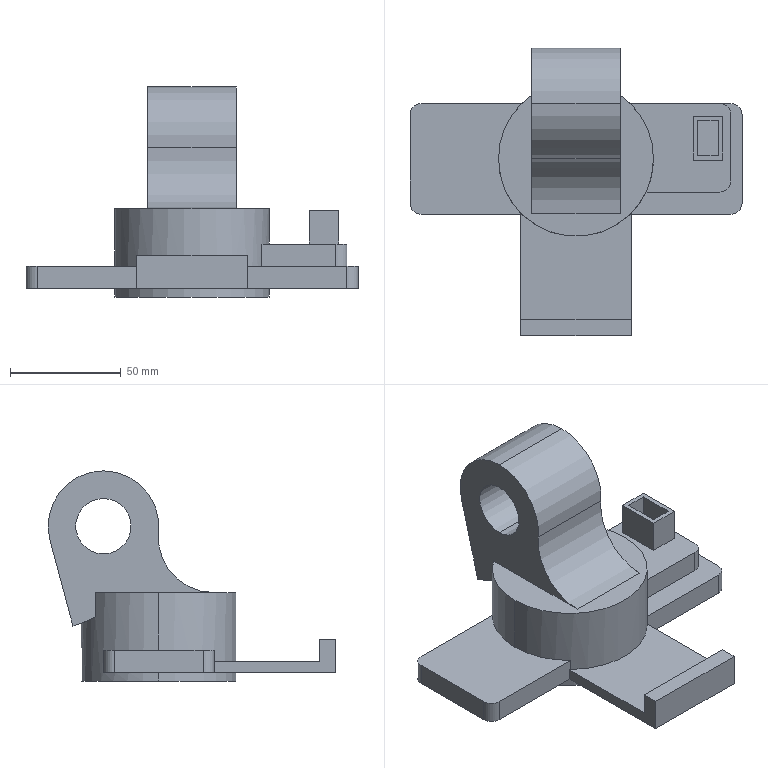Part | SolidWorks | features ICE 6, Fillet 4, Cut 2, Extrusion 1 | 1 solid | 48 faces | box 150 x 130 x 95 mm | volume 315540 mm3 | plane 33 | cylinder 15 | commonest cylinder face diameters 10 x6 50 x3 70 x3 25 x2 80 x1
STEP:
#1=CARTESIAN_POINT('',(-20.,25.,82.5));
#2=VERTEX_POINT('',#1);
#3=CARTESIAN_POINT('',(-20.,25.,57.5));
#4=VERTEX_POINT('',#3);
#5=CARTESIAN_POINT('',(-20.,25.,70.));
#6=DIRECTION('',(1.,0.,0.));
#7=DIRECTION('',(0.,0.,-1.));
#8=AXIS2_PLACEMENT_3D('',#5,#6,#7);
#9=CIRCLE('',#8,12.5);
#10=EDGE_CURVE('',#2,#4,#9,.T.);
#11=ORIENTED_EDGE('',*,*,#10,.F.);
#12=CARTESIAN_POINT('',(20.,25.,82.5));
#13=VERTEX_POINT('',#12);
#14=CARTESIAN_POINT('',(-75.,25.,82.5));
#15=DIRECTION('',(1.,0.,0.));
#16=VECTOR('',#15,1000.);
#17=LINE('',#14,#16);
#18=EDGE_CURVE('',#2,#13,#17,.T.);
#19=ORIENTED_EDGE('',*,*,#18,.T.);
#20=CARTESIAN_POINT('',(20.,25.,57.5));
#21=VERTEX_POINT('',#20);
#22=CARTESIAN_POINT('',(20.,25.,70.));
#23=DIRECTION('',(1.,0.,0.));
#24=DIRECTION('',(0.,0.,-1.));
#25=AXIS2_PLACEMENT_3D('',#22,#23,#24);
#26=CIRCLE('',#25,12.5);
#27=EDGE_CURVE('',#13,#21,#26,.T.);
#28=ORIENTED_EDGE('',*,*,#27,.T.);
#29=CARTESIAN_POINT('',(-75.,25.,57.5));
#30=DIRECTION('',(1.,0.,0.));
#31=VECTOR('',#30,1000.);
#32=LINE('',#29,#31);
#33=EDGE_CURVE('',#4,#21,#32,.T.);
#34=ORIENTED_EDGE('',*,*,#33,.F.);
#35=EDGE_LOOP('',(#11,#19,#28,#34));
#36=FACE_OUTER_BOUND('',#35,.T.);
#37=CARTESIAN_POINT('',(-75.,25.,70.));
#38=DIRECTION('',(1.,0.,0.));
#39=DIRECTION('',(0.,0.,-1.));
#40=AXIS2_PLACEMENT_3D('',#37,#38,#39);
#41=CYLINDRICAL_SURFACE('',#40,12.5);
#42=ADVANCED_FACE('',(#36),#41,.F.);
#43=CARTESIAN_POINT('',(20.,25.,95.));
#44=VERTEX_POINT('',#43);
#45=CARTESIAN_POINT('',(20.,0.1253,67.5));
#46=VERTEX_POINT('',#45);
#47=CARTESIAN_POINT('',(20.,25.,70.));
#48=DIRECTION('',(1.,0.,0.));
#49=DIRECTION('',(0.,0.,-1.));
#50=AXIS2_PLACEMENT_3D('',#47,#48,#49);
#51=CIRCLE('',#50,25.);
#52=EDGE_CURVE('',#44,#46,#51,.T.);
#53=ORIENTED_EDGE('',*,*,#52,.F.);
#54=CARTESIAN_POINT('',(-20.,25.,95.));
#55=VERTEX_POINT('',#54);
#56=CARTESIAN_POINT('',(20.,25.,95.));
#57=DIRECTION('',(-1.,0.,0.));
#58=VECTOR('',#57,1000.);
#59=LINE('',#56,#58);
#60=EDGE_CURVE('',#44,#55,#59,.T.);
#61=ORIENTED_EDGE('',*,*,#60,.T.);
#62=CARTESIAN_POINT('',(-20.,0.1253,67.5));
#63=VERTEX_POINT('',#62);
#64=CARTESIAN_POINT('',(-20.,25.,70.));
#65=DIRECTION('',(1.,0.,0.));
#66=DIRECTION('',(0.,0.,-1.));
#67=AXIS2_PLACEMENT_3D('',#64,#65,#66);
#68=CIRCLE('',#67,25.);
#69=EDGE_CURVE('',#55,#63,#68,.T.);
#70=ORIENTED_EDGE('',*,*,#69,.T.);
#71=CARTESIAN_POINT('',(20.,0.1253,67.5));
#72=DIRECTION('',(1.,0.,0.));
#73=VECTOR('',#72,1000.);
#74=LINE('',#71,#73);
#75=EDGE_CURVE('',#63,#46,#74,.T.);
#76=ORIENTED_EDGE('',*,*,#75,.T.);
#77=EDGE_LOOP('',(#53,#61,#70,#76));
#78=FACE_OUTER_BOUND('',#77,.T.);
#79=CARTESIAN_POINT('',(20.,25.,70.));
#80=DIRECTION('',(-1.,0.,0.));
#81=DIRECTION('',(0.,0.,1.));
#82=AXIS2_PLACEMENT_3D('',#79,#80,#81);
#83=CYLINDRICAL_SURFACE('',#82,25.);
#84=ADVANCED_FACE('',(#78),#83,.T.);
#85=CARTESIAN_POINT('',(35.,0.,40.));
#86=VERTEX_POINT('',#85);
#87=CARTESIAN_POINT('',(20.,28.723,40.));
#88=VERTEX_POINT('',#87);
#89=CARTESIAN_POINT('',(0.,0.,40.));
#90=DIRECTION('',(0.,0.,1.));
#91=DIRECTION('',(1.,0.,0.));
#92=AXIS2_PLACEMENT_3D('',#89,#90,#91);
#93=CIRCLE('',#92,35.);
#94=EDGE_CURVE('',#86,#88,#93,.T.);
#95=ORIENTED_EDGE('',*,*,#94,.F.);
#96=CARTESIAN_POINT('',(35.,0.,24.));
#97=VERTEX_POINT('',#96);
#98=CARTESIAN_POINT('',(35.,0.,40.));
#99=DIRECTION('',(0.,0.,-1.));
#100=VECTOR('',#99,1000.);
#101=LINE('',#98,#100);
#102=EDGE_CURVE('',#86,#97,#101,.T.);
#103=ORIENTED_EDGE('',*,*,#102,.T.);
#104=CARTESIAN_POINT('',(24.495,25.,24.));
#105=VERTEX_POINT('',#104);
#106=CARTESIAN_POINT('',(0.,0.,24.));
#107=DIRECTION('',(0.,0.,-1.));
#108=DIRECTION('',(0.,1.,0.));
#109=AXIS2_PLACEMENT_3D('',#106,#107,#108);
#110=CIRCLE('',#109,35.);
#111=EDGE_CURVE('',#105,#97,#110,.T.);
#112=ORIENTED_EDGE('',*,*,#111,.F.);
#113=CARTESIAN_POINT('',(24.495,25.,4.));
#114=VERTEX_POINT('',#113);
#115=CARTESIAN_POINT('',(24.495,25.,40.));
#116=DIRECTION('',(0.,0.,1.));
#117=VECTOR('',#116,1000.);
#118=LINE('',#115,#117);
#119=EDGE_CURVE('',#114,#105,#118,.T.);
#120=ORIENTED_EDGE('',*,*,#119,.F.);
#121=CARTESIAN_POINT('',(35.,0.,4.));
#122=VERTEX_POINT('',#121);
#123=CARTESIAN_POINT('',(0.,0.,4.));
#124=DIRECTION('',(0.,0.,-1.));
#125=DIRECTION('',(-1.,0.,0.));
#126=AXIS2_PLACEMENT_3D('',#123,#124,#125);
#127=CIRCLE('',#126,35.);
#128=EDGE_CURVE('',#114,#122,#127,.T.);
#129=ORIENTED_EDGE('',*,*,#128,.T.);
#130=CARTESIAN_POINT('',(35.,0.,0.));
#131=VERTEX_POINT('',#130);
#132=CARTESIAN_POINT('',(35.,0.,40.));
#133=DIRECTION('',(0.,0.,-1.));
#134=VECTOR('',#133,1000.);
#135=LINE('',#132,#134);
#136=EDGE_CURVE('',#122,#131,#135,.T.);
#137=ORIENTED_EDGE('',*,*,#136,.T.);
#138=CARTESIAN_POINT('',(-35.,0.,0.));
#139=VERTEX_POINT('',#138);
#140=CARTESIAN_POINT('',(0.,0.,0.));
#141=DIRECTION('',(0.,0.,1.));
#142=DIRECTION('',(1.,0.,0.));
#143=AXIS2_PLACEMENT_3D('',#140,#141,#142);
#144=CIRCLE('',#143,35.);
#145=EDGE_CURVE('',#131,#139,#144,.T.);
#146=ORIENTED_EDGE('',*,*,#145,.T.);
#147=CARTESIAN_POINT('',(-35.,0.,4.));
#148=VERTEX_POINT('',#147);
#149=CARTESIAN_POINT('',(-35.,0.,40.));
#150=DIRECTION('',(0.,0.,-1.));
#151=VECTOR('',#150,1000.);
#152=LINE('',#149,#151);
#153=EDGE_CURVE('',#148,#139,#152,.T.);
#154=ORIENTED_EDGE('',*,*,#153,.F.);
#155=CARTESIAN_POINT('',(-24.495,25.,4.));
#156=VERTEX_POINT('',#155);
#157=CARTESIAN_POINT('',(0.,0.,4.));
#158=DIRECTION('',(0.,0.,-1.));
#159=DIRECTION('',(-1.,0.,0.));
#160=AXIS2_PLACEMENT_3D('',#157,#158,#159);
#161=CIRCLE('',#160,35.);
#162=EDGE_CURVE('',#148,#156,#161,.T.);
#163=ORIENTED_EDGE('',*,*,#162,.T.);
#164=CARTESIAN_POINT('',(-24.495,25.,14.));
#165=VERTEX_POINT('',#164);
#166=CARTESIAN_POINT('',(-24.495,25.,40.));
#167=DIRECTION('',(0.,0.,-1.));
#168=VECTOR('',#167,1000.);
#169=LINE('',#166,#168);
#170=EDGE_CURVE('',#165,#156,#169,.T.);
#171=ORIENTED_EDGE('',*,*,#170,.F.);
#172=CARTESIAN_POINT('',(-35.,0.,14.));
#173=VERTEX_POINT('',#172);
#174=CARTESIAN_POINT('',(0.,0.,14.));
#175=DIRECTION('',(0.,0.,-1.));
#176=DIRECTION('',(0.,1.,0.));
#177=AXIS2_PLACEMENT_3D('',#174,#175,#176);
#178=CIRCLE('',#177,35.);
#179=EDGE_CURVE('',#173,#165,#178,.T.);
#180=ORIENTED_EDGE('',*,*,#179,.F.);
#181=CARTESIAN_POINT('',(-35.,0.,40.));
#182=VERTEX_POINT('',#181);
#183=CARTESIAN_POINT('',(-35.,0.,40.));
#184=DIRECTION('',(0.,0.,-1.));
#185=VECTOR('',#184,1000.);
#186=LINE('',#183,#185);
#187=EDGE_CURVE('',#182,#173,#186,.T.);
#188=ORIENTED_EDGE('',*,*,#187,.F.);
#189=CARTESIAN_POINT('',(-20.,28.723,40.));
#190=VERTEX_POINT('',#189);
#191=CARTESIAN_POINT('',(0.,0.,40.));
#192=DIRECTION('',(0.,0.,1.));
#193=DIRECTION('',(1.,0.,0.));
#194=AXIS2_PLACEMENT_3D('',#191,#192,#193);
#195=CIRCLE('',#194,35.);
#196=EDGE_CURVE('',#190,#182,#195,.T.);
#197=ORIENTED_EDGE('',*,*,#196,.F.);
#198=CARTESIAN_POINT('',(-20.,28.723,29.138));
#199=VERTEX_POINT('',#198);
#200=CARTESIAN_POINT('',(-20.,28.723,40.));
#201=DIRECTION('',(0.,0.,1.));
#202=VECTOR('',#201,1000.);
#203=LINE('',#200,#202);
#204=EDGE_CURVE('',#199,#190,#203,.T.);
#205=ORIENTED_EDGE('',*,*,#204,.F.);
#206=CARTESIAN_POINT('',(20.,28.723,29.138));
#207=VERTEX_POINT('',#206);
#208=CARTESIAN_POINT('',(20.,28.723,29.138));
#209=CARTESIAN_POINT('',(19.295,29.214,28.846));
#210=CARTESIAN_POINT('',(18.566,29.682,28.582));
#211=CARTESIAN_POINT('',(17.074,30.565,28.105));
#212=CARTESIAN_POINT('',(16.308,30.981,27.89));
#213=CARTESIAN_POINT('',(14.738,31.758,27.505));
#214=CARTESIAN_POINT('',(13.933,32.119,27.333));
#215=CARTESIAN_POINT('',(12.286,32.785,27.028));
#216=CARTESIAN_POINT('',(11.439,33.09,26.893));
#217=CARTESIAN_POINT('',(8.876,33.903,26.544));
#218=CARTESIAN_POINT('',(7.136,34.312,26.382));
#219=CARTESIAN_POINT('',(4.482,34.723,26.221));
#220=CARTESIAN_POINT('',(3.589,34.827,26.181));
#221=CARTESIAN_POINT('',(1.79,34.966,26.128));
#222=CARTESIAN_POINT('',(0.8798,35.001,26.115));
#223=CARTESIAN_POINT('',(-1.825,34.999,26.116));
#224=CARTESIAN_POINT('',(-3.61,34.859,26.168));
#225=CARTESIAN_POINT('',(-6.261,34.447,26.329));
#226=CARTESIAN_POINT('',(-7.14,34.276,26.397));
#227=CARTESIAN_POINT('',(-8.89,33.864,26.564));
#228=CARTESIAN_POINT('',(-9.762,33.623,26.664));
#229=CARTESIAN_POINT('',(-12.318,32.809,27.014));
#230=CARTESIAN_POINT('',(-13.954,32.146,27.313));
#231=CARTESIAN_POINT('',(-16.303,30.984,27.889));
#232=CARTESIAN_POINT('',(-17.069,30.568,28.103));
#233=CARTESIAN_POINT('',(-18.565,29.683,28.581));
#234=CARTESIAN_POINT('',(-19.298,29.211,28.847));
#235=CARTESIAN_POINT('',(-20.,28.723,29.138));
#236=B_SPLINE_CURVE_WITH_KNOTS('',3,(#208,#209,#210,#211,#212,#213,#214,#215,#216,#217,#218,#219,#220,#221,#222,#223,#224,#225,#226,#227,#228,#229,#230,#231,#232,#233,#234,#235),.UNSPECIFIED.,.F.,.F.,(4,2,2,2,2,2,2,2,2,2,2,2,2,4),(0.01965,0.02233,0.02502,0.02771,0.03039,0.03577,0.03846,0.04114,0.04652,0.0492,0.05189,0.05726,0.05995,0.06264),.UNSPECIFIED.);
#237=EDGE_CURVE('',#207,#199,#236,.T.);
#238=ORIENTED_EDGE('',*,*,#237,.F.);
#239=CARTESIAN_POINT('',(20.,28.723,40.));
#240=DIRECTION('',(0.,0.,1.));
#241=VECTOR('',#240,1000.);
#242=LINE('',#239,#241);
#243=EDGE_CURVE('',#207,#88,#242,.T.);
#244=ORIENTED_EDGE('',*,*,#243,.T.);
#245=EDGE_LOOP('',(#95,#103,#112,#120,#129,#137,#146,#154,#163,#171,#180,#188,#197,#205,#238,#244));
#246=FACE_OUTER_BOUND('',#245,.T.);
#247=CARTESIAN_POINT('',(0.,0.,40.));
#248=DIRECTION('',(0.,0.,-1.));
#249=DIRECTION('',(-1.,0.,0.));
#250=AXIS2_PLACEMENT_3D('',#247,#248,#249);
#251=CYLINDRICAL_SURFACE('',#250,35.);
#252=ADVANCED_FACE('',(#246),#251,.T.);
#253=ORIENTED_EDGE('',*,*,#102,.F.);
#254=CARTESIAN_POINT('',(0.,0.,40.));
#255=DIRECTION('',(0.,0.,1.));
#256=DIRECTION('',(1.,0.,0.));
#257=AXIS2_PLACEMENT_3D('',#254,#255,#256);
#258=CIRCLE('',#257,35.);
#259=EDGE_CURVE('',#182,#86,#258,.T.);
#260=ORIENTED_EDGE('',*,*,#259,.F.);
#261=ORIENTED_EDGE('',*,*,#187,.T.);
#262=CARTESIAN_POINT('',(-24.495,-25.,14.));
#263=VERTEX_POINT('',#262);
#264=CARTESIAN_POINT('',(0.,0.,14.));
#265=DIRECTION('',(0.,0.,-1.));
#266=DIRECTION('',(0.,1.,0.));
#267=AXIS2_PLACEMENT_3D('',#264,#265,#266);
#268=CIRCLE('',#267,35.);
#269=EDGE_CURVE('',#263,#173,#268,.T.);
#270=ORIENTED_EDGE('',*,*,#269,.F.);
#271=CARTESIAN_POINT('',(-24.495,-25.,9.));
#272=VERTEX_POINT('',#271);
#273=CARTESIAN_POINT('',(-24.495,-25.,40.));
#274=DIRECTION('',(0.,0.,1.));
#275=VECTOR('',#274,1000.);
#276=LINE('',#273,#275);
#277=EDGE_CURVE('',#272,#263,#276,.T.);
#278=ORIENTED_EDGE('',*,*,#277,.F.);
#279=CARTESIAN_POINT('',(24.495,-25.,9.));
#280=VERTEX_POINT('',#279);
#281=CARTESIAN_POINT('',(0.,0.,9.));
#282=DIRECTION('',(0.,0.,1.));
#283=DIRECTION('',(1.,0.,0.));
#284=AXIS2_PLACEMENT_3D('',#281,#282,#283);
#285=CIRCLE('',#284,35.);
#286=EDGE_CURVE('',#272,#280,#285,.T.);
#287=ORIENTED_EDGE('',*,*,#286,.T.);
#288=CARTESIAN_POINT('',(24.495,-25.,14.));
#289=VERTEX_POINT('',#288);
#290=CARTESIAN_POINT('',(24.495,-25.,40.));
#291=DIRECTION('',(0.,0.,-1.));
#292=VECTOR('',#291,1000.);
#293=LINE('',#290,#292);
#294=EDGE_CURVE('',#289,#280,#293,.T.);
#295=ORIENTED_EDGE('',*,*,#294,.F.);
#296=CARTESIAN_POINT('',(31.623,-15.,14.));
#297=VERTEX_POINT('',#296);
#298=CARTESIAN_POINT('',(0.,0.,14.));
#299=DIRECTION('',(0.,0.,-1.));
#300=DIRECTION('',(0.,1.,0.));
#301=AXIS2_PLACEMENT_3D('',#298,#299,#300);
#302=CIRCLE('',#301,35.);
#303=EDGE_CURVE('',#297,#289,#302,.T.);
#304=ORIENTED_EDGE('',*,*,#303,.F.);
#305=CARTESIAN_POINT('',(31.623,-15.,24.));
#306=VERTEX_POINT('',#305);
#307=CARTESIAN_POINT('',(31.623,-15.,40.));
#308=DIRECTION('',(0.,0.,-1.));
#309=VECTOR('',#308,1000.);
#310=LINE('',#307,#309);
#311=EDGE_CURVE('',#306,#297,#310,.T.);
#312=ORIENTED_EDGE('',*,*,#311,.F.);
#313=CARTESIAN_POINT('',(0.,0.,24.));
#314=DIRECTION('',(0.,0.,-1.));
#315=DIRECTION('',(0.,1.,0.));
#316=AXIS2_PLACEMENT_3D('',#313,#314,#315);
#317=CIRCLE('',#316,35.);
#318=EDGE_CURVE('',#97,#306,#317,.T.);
#319=ORIENTED_EDGE('',*,*,#318,.F.);
#320=EDGE_LOOP('',(#253,#260,#261,#270,#278,#287,#295,#304,#312,#319));
#321=FACE_OUTER_BOUND('',#320,.T.);
#322=CARTESIAN_POINT('',(0.,0.,40.));
#323=DIRECTION('',(0.,0.,-1.));
#324=DIRECTION('',(-1.,0.,0.));
#325=AXIS2_PLACEMENT_3D('',#322,#323,#324);
#326=CYLINDRICAL_SURFACE('',#325,35.);
#327=ADVANCED_FACE('',(#321),#326,.T.);
#328=CARTESIAN_POINT('',(65.,-15.,24.));
#329=VERTEX_POINT('',#328);
#330=CARTESIAN_POINT('',(70.,-15.,24.));
#331=DIRECTION('',(-1.,0.,0.));
#332=VECTOR('',#331,1000.);
#333=LINE('',#330,#332);
#334=EDGE_CURVE('',#329,#306,#333,.T.);
#335=ORIENTED_EDGE('',*,*,#334,.F.);
#336=CARTESIAN_POINT('',(70.,-10.,24.));
#337=VERTEX_POINT('',#336);
#338=CARTESIAN_POINT('',(65.,-10.,24.));
#339=DIRECTION('',(0.,0.,1.));
#340=DIRECTION('',(0.,1.,0.));
#341=AXIS2_PLACEMENT_3D('',#338,#339,#340);
#342=CIRCLE('',#341,5.);
#343=EDGE_CURVE('',#329,#337,#342,.T.);
#344=ORIENTED_EDGE('',*,*,#343,.T.);
#345=CARTESIAN_POINT('',(70.,20.,24.));
#346=VERTEX_POINT('',#345);
#347=CARTESIAN_POINT('',(70.,25.,24.));
#348=DIRECTION('',(0.,-1.,0.));
#349=VECTOR('',#348,1000.);
#350=LINE('',#347,#349);
#351=EDGE_CURVE('',#346,#337,#350,.T.);
#352=ORIENTED_EDGE('',*,*,#351,.F.);
#353=CARTESIAN_POINT('',(65.,25.,24.));
#354=VERTEX_POINT('',#353);
#355=CARTESIAN_POINT('',(65.,20.,24.));
#356=DIRECTION('',(0.,0.,1.));
#357=DIRECTION('',(0.,1.,0.));
#358=AXIS2_PLACEMENT_3D('',#355,#356,#357);
#359=CIRCLE('',#358,5.);
#360=EDGE_CURVE('',#346,#354,#359,.T.);
#361=ORIENTED_EDGE('',*,*,#360,.T.);
#362=CARTESIAN_POINT('',(70.,25.,24.));
#363=DIRECTION('',(-1.,0.,0.));
#364=VECTOR('',#363,1000.);
#365=LINE('',#362,#364);
#366=EDGE_CURVE('',#354,#105,#365,.T.);
#367=ORIENTED_EDGE('',*,*,#366,.T.);
#368=ORIENTED_EDGE('',*,*,#111,.T.);
#369=ORIENTED_EDGE('',*,*,#318,.T.);
#370=EDGE_LOOP('',(#335,#344,#352,#361,#367,#368,#369));
#371=FACE_OUTER_BOUND('',#370,.T.);
#372=CARTESIAN_POINT('',(52.886,19.241,24.));
#373=VERTEX_POINT('',#372);
#374=CARTESIAN_POINT('',(52.886,-0.6252,24.));
#375=VERTEX_POINT('',#374);
#376=CARTESIAN_POINT('',(52.886,19.241,24.));
#377=DIRECTION('',(0.,-1.,0.));
#378=VECTOR('',#377,1000.);
#379=LINE('',#376,#378);
#380=EDGE_CURVE('',#373,#375,#379,.T.);
#381=ORIENTED_EDGE('',*,*,#380,.F.);
#382=CARTESIAN_POINT('',(66.302,19.241,24.));
#383=VERTEX_POINT('',#382);
#384=CARTESIAN_POINT('',(66.302,19.241,24.));
#385=DIRECTION('',(-1.,0.,0.));
#386=VECTOR('',#385,1000.);
#387=LINE('',#384,#386);
#388=EDGE_CURVE('',#383,#373,#387,.T.);
#389=ORIENTED_EDGE('',*,*,#388,.F.);
#390=CARTESIAN_POINT('',(66.302,-0.6252,24.));
#391=VERTEX_POINT('',#390);
#392=CARTESIAN_POINT('',(66.302,19.241,24.));
#393=DIRECTION('',(0.,1.,0.));
#394=VECTOR('',#393,1000.);
#395=LINE('',#392,#394);
#396=EDGE_CURVE('',#391,#383,#395,.T.);
#397=ORIENTED_EDGE('',*,*,#396,.F.);
#398=CARTESIAN_POINT('',(66.302,-0.6252,24.));
#399=DIRECTION('',(1.,0.,0.));
#400=VECTOR('',#399,1000.);
#401=LINE('',#398,#400);
#402=EDGE_CURVE('',#375,#391,#401,.T.);
#403=ORIENTED_EDGE('',*,*,#402,.F.);
#404=EDGE_LOOP('',(#381,#389,#397,#403));
#405=FACE_BOUND('',#404,.T.);
#406=CARTESIAN_POINT('',(70.,25.,24.));
#407=DIRECTION('',(0.,0.,-1.));
#408=DIRECTION('',(0.,1.,0.));
#409=AXIS2_PLACEMENT_3D('',#406,#407,#408);
#410=PLANE('',#409);
#411=ADVANCED_FACE('',(#371,#405),#410,.F.);
#412=ORIENTED_EDGE('',*,*,#136,.F.);
#413=CARTESIAN_POINT('',(0.,0.,4.));
#414=DIRECTION('',(0.,0.,-1.));
#415=DIRECTION('',(-1.,0.,0.));
#416=AXIS2_PLACEMENT_3D('',#413,#414,#415);
#417=CIRCLE('',#416,35.);
#418=EDGE_CURVE('',#122,#148,#417,.T.);
#419=ORIENTED_EDGE('',*,*,#418,.T.);
#420=ORIENTED_EDGE('',*,*,#153,.T.);
#421=CARTESIAN_POINT('',(0.,0.,0.));
#422=DIRECTION('',(0.,0.,1.));
#423=DIRECTION('',(1.,0.,0.));
#424=AXIS2_PLACEMENT_3D('',#421,#422,#423);
#425=CIRCLE('',#424,35.);
#426=EDGE_CURVE('',#139,#131,#425,.T.);
#427=ORIENTED_EDGE('',*,*,#426,.T.);
#428=EDGE_LOOP('',(#412,#419,#420,#427));
#429=FACE_OUTER_BOUND('',#428,.T.);
#430=CARTESIAN_POINT('',(0.,0.,40.));
#431=DIRECTION('',(0.,0.,-1.));
#432=DIRECTION('',(-1.,0.,0.));
#433=AXIS2_PLACEMENT_3D('',#430,#431,#432);
#434=CYLINDRICAL_SURFACE('',#433,35.);
#435=ADVANCED_FACE('',(#429),#434,.T.);
#436=CARTESIAN_POINT('',(70.,-25.,14.));
#437=VERTEX_POINT('',#436);
#438=CARTESIAN_POINT('',(75.,-25.,14.));
#439=DIRECTION('',(-1.,0.,0.));
#440=VECTOR('',#439,1000.);
#441=LINE('',#438,#440);
#442=EDGE_CURVE('',#437,#289,#441,.T.);
#443=ORIENTED_EDGE('',*,*,#442,.F.);
#444=CARTESIAN_POINT('',(75.,-20.,14.));
#445=VERTEX_POINT('',#444);
#446=CARTESIAN_POINT('',(70.,-20.,14.));
#447=DIRECTION('',(0.,0.,1.));
#448=DIRECTION('',(0.,1.,0.));
#449=AXIS2_PLACEMENT_3D('',#446,#447,#448);
#450=CIRCLE('',#449,5.);
#451=EDGE_CURVE('',#437,#445,#450,.T.);
#452=ORIENTED_EDGE('',*,*,#451,.T.);
#453=CARTESIAN_POINT('',(75.,20.,14.));
#454=VERTEX_POINT('',#453);
#455=CARTESIAN_POINT('',(75.,25.,14.));
#456=DIRECTION('',(0.,-1.,0.));
#457=VECTOR('',#456,1000.);
#458=LINE('',#455,#457);
#459=EDGE_CURVE('',#454,#445,#458,.T.);
#460=ORIENTED_EDGE('',*,*,#459,.F.);
#461=CARTESIAN_POINT('',(70.,25.,14.));
#462=VERTEX_POINT('',#461);
#463=CARTESIAN_POINT('',(70.,20.,14.));
#464=DIRECTION('',(0.,0.,1.));
#465=DIRECTION('',(0.,1.,0.));
#466=AXIS2_PLACEMENT_3D('',#463,#464,#465);
#467=CIRCLE('',#466,5.);
#468=EDGE_CURVE('',#454,#462,#467,.T.);
#469=ORIENTED_EDGE('',*,*,#468,.T.);
#470=CARTESIAN_POINT('',(65.,25.,14.));
#471=VERTEX_POINT('',#470);
#472=CARTESIAN_POINT('',(75.,25.,14.));
#473=DIRECTION('',(1.,0.,0.));
#474=VECTOR('',#473,1000.);
#475=LINE('',#472,#474);
#476=EDGE_CURVE('',#471,#462,#475,.T.);
#477=ORIENTED_EDGE('',*,*,#476,.F.);
#478=CARTESIAN_POINT('',(70.,20.,14.));
#479=VERTEX_POINT('',#478);
#480=CARTESIAN_POINT('',(65.,20.,14.));
#481=DIRECTION('',(0.,0.,-1.));
#482=DIRECTION('',(0.,1.,0.));
#483=AXIS2_PLACEMENT_3D('',#480,#481,#482);
#484=CIRCLE('',#483,5.);
#485=EDGE_CURVE('',#471,#479,#484,.T.);
#486=ORIENTED_EDGE('',*,*,#485,.T.);
#487=CARTESIAN_POINT('',(70.,-10.,14.));
#488=VERTEX_POINT('',#487);
#489=CARTESIAN_POINT('',(70.,25.,14.));
#490=DIRECTION('',(0.,1.,0.));
#491=VECTOR('',#490,1000.);
#492=LINE('',#489,#491);
#493=EDGE_CURVE('',#488,#479,#492,.T.);
#494=ORIENTED_EDGE('',*,*,#493,.F.);
#495=CARTESIAN_POINT('',(65.,-15.,14.));
#496=VERTEX_POINT('',#495);
#497=CARTESIAN_POINT('',(65.,-10.,14.));
#498=DIRECTION('',(0.,0.,-1.));
#499=DIRECTION('',(0.,1.,0.));
#500=AXIS2_PLACEMENT_3D('',#497,#498,#499);
#501=CIRCLE('',#500,5.);
#502=EDGE_CURVE('',#488,#496,#501,.T.);
#503=ORIENTED_EDGE('',*,*,#502,.T.);
#504=CARTESIAN_POINT('',(70.,-15.,14.));
#505=DIRECTION('',(-1.,0.,0.));
#506=VECTOR('',#505,1000.);
#507=LINE('',#504,#506);
#508=EDGE_CURVE('',#496,#297,#507,.T.);
#509=ORIENTED_EDGE('',*,*,#508,.T.);
#510=ORIENTED_EDGE('',*,*,#303,.T.);
#511=EDGE_LOOP('',(#443,#452,#460,#469,#477,#486,#494,#503,#509,#510));
#512=FACE_OUTER_BOUND('',#511,.T.);
#513=CARTESIAN_POINT('',(75.,25.,14.));
#514=DIRECTION('',(0.,0.,-1.));
#515=DIRECTION('',(0.,1.,0.));
#516=AXIS2_PLACEMENT_3D('',#513,#514,#515);
#517=PLANE('',#516);
#518=ADVANCED_FACE('',(#512),#517,.F.);
#519=CARTESIAN_POINT('',(25.,-72.5,9.));
#520=VERTEX_POINT('',#519);
#521=CARTESIAN_POINT('',(25.,-25.,9.));
#522=VERTEX_POINT('',#521);
#523=CARTESIAN_POINT('',(25.,-80.,9.));
#524=DIRECTION('',(0.,1.,0.));
#525=VECTOR('',#524,1000.);
#526=LINE('',#523,#525);
#527=EDGE_CURVE('',#520,#522,#526,.T.);
#528=ORIENTED_EDGE('',*,*,#527,.T.);
#529=CARTESIAN_POINT('',(-25.,-25.,9.));
#530=DIRECTION('',(-1.,0.,0.));
#531=VECTOR('',#530,1000.);
#532=LINE('',#529,#531);
#533=EDGE_CURVE('',#522,#280,#532,.T.);
#534=ORIENTED_EDGE('',*,*,#533,.T.);
#535=ORIENTED_EDGE('',*,*,#286,.F.);
#536=CARTESIAN_POINT('',(-25.,-25.,9.));
#537=VERTEX_POINT('',#536);
#538=CARTESIAN_POINT('',(-25.,-25.,9.));
#539=DIRECTION('',(-1.,0.,0.));
#540=VECTOR('',#539,1000.);
#541=LINE('',#538,#540);
#542=EDGE_CURVE('',#272,#537,#541,.T.);
#543=ORIENTED_EDGE('',*,*,#542,.T.);
#544=CARTESIAN_POINT('',(-25.,-72.5,9.));
#545=VERTEX_POINT('',#544);
#546=CARTESIAN_POINT('',(-25.,-80.,9.));
#547=DIRECTION('',(0.,1.,0.));
#548=VECTOR('',#547,1000.);
#549=LINE('',#546,#548);
#550=EDGE_CURVE('',#545,#537,#549,.T.);
#551=ORIENTED_EDGE('',*,*,#550,.F.);
#552=CARTESIAN_POINT('',(25.,-72.5,9.));
#553=DIRECTION('',(-1.,0.,0.));
#554=VECTOR('',#553,1000.);
#555=LINE('',#552,#554);
#556=EDGE_CURVE('',#520,#545,#555,.T.);
#557=ORIENTED_EDGE('',*,*,#556,.F.);
#558=EDGE_LOOP('',(#528,#534,#535,#543,#551,#557));
#559=FACE_OUTER_BOUND('',#558,.T.);
#560=CARTESIAN_POINT('',(-25.,-80.,9.));
#561=DIRECTION('',(0.,0.,1.));
#562=DIRECTION('',(1.,0.,0.));
#563=AXIS2_PLACEMENT_3D('',#560,#561,#562);
#564=PLANE('',#563);
#565=ADVANCED_FACE('',(#559),#564,.T.);
#566=CARTESIAN_POINT('',(25.,-80.,4.));
#567=VERTEX_POINT('',#566);
#568=CARTESIAN_POINT('',(25.,-25.,4.));
#569=VERTEX_POINT('',#568);
#570=CARTESIAN_POINT('',(25.,-80.,4.));
#571=DIRECTION('',(0.,1.,0.));
#572=VECTOR('',#571,1000.);
#573=LINE('',#570,#572);
#574=EDGE_CURVE('',#567,#569,#573,.T.);
#575=ORIENTED_EDGE('',*,*,#574,.T.);
#576=CARTESIAN_POINT('',(25.,-25.,4.));
#577=DIRECTION('',(0.,0.,1.));
#578=VECTOR('',#577,1000.);
#579=LINE('',#576,#578);
#580=EDGE_CURVE('',#569,#522,#579,.T.);
#581=ORIENTED_EDGE('',*,*,#580,.T.);
#582=ORIENTED_EDGE('',*,*,#527,.F.);
#583=CARTESIAN_POINT('',(25.,-72.5,19.));
#584=VERTEX_POINT('',#583);
#585=CARTESIAN_POINT('',(25.,-72.5,19.));
#586=DIRECTION('',(0.,0.,-1.));
#587=VECTOR('',#586,1000.);
#588=LINE('',#585,#587);
#589=EDGE_CURVE('',#584,#520,#588,.T.);
#590=ORIENTED_EDGE('',*,*,#589,.F.);
#591=CARTESIAN_POINT('',(25.,-80.,19.));
#592=VERTEX_POINT('',#591);
#593=CARTESIAN_POINT('',(25.,-80.,19.));
#594=DIRECTION('',(0.,1.,0.));
#595=VECTOR('',#594,1000.);
#596=LINE('',#593,#595);
#597=EDGE_CURVE('',#592,#584,#596,.T.);
#598=ORIENTED_EDGE('',*,*,#597,.F.);
#599=CARTESIAN_POINT('',(25.,-80.,4.));
#600=DIRECTION('',(0.,0.,-1.));
#601=VECTOR('',#600,1000.);
#602=LINE('',#599,#601);
#603=EDGE_CURVE('',#592,#567,#602,.T.);
#604=ORIENTED_EDGE('',*,*,#603,.T.);
#605=EDGE_LOOP('',(#575,#581,#582,#590,#598,#604));
#606=FACE_OUTER_BOUND('',#605,.T.);
#607=CARTESIAN_POINT('',(25.,-80.,4.));
#608=DIRECTION('',(1.,0.,0.));
#609=DIRECTION('',(0.,0.,-1.));
#610=AXIS2_PLACEMENT_3D('',#607,#608,#609);
#611=PLANE('',#610);
#612=ADVANCED_FACE('',(#606),#611,.T.);
#613=ORIENTED_EDGE('',*,*,#550,.T.);
#614=CARTESIAN_POINT('',(-25.,-25.,4.));
#615=VERTEX_POINT('',#614);
#616=CARTESIAN_POINT('',(-25.,-25.,4.));
#617=DIRECTION('',(0.,0.,-1.));
#618=VECTOR('',#617,1000.);
#619=LINE('',#616,#618);
#620=EDGE_CURVE('',#537,#615,#619,.T.);
#621=ORIENTED_EDGE('',*,*,#620,.T.);
#622=CARTESIAN_POINT('',(-25.,-80.,4.));
#623=VERTEX_POINT('',#622);
#624=CARTESIAN_POINT('',(-25.,-80.,4.));
#625=DIRECTION('',(0.,1.,0.));
#626=VECTOR('',#625,1000.);
#627=LINE('',#624,#626);
#628=EDGE_CURVE('',#623,#615,#627,.T.);
#629=ORIENTED_EDGE('',*,*,#628,.F.);
#630=CARTESIAN_POINT('',(-25.,-80.,19.));
#631=VERTEX_POINT('',#630);
#632=CARTESIAN_POINT('',(-25.,-80.,4.));
#633=DIRECTION('',(0.,0.,1.));
#634=VECTOR('',#633,1000.);
#635=LINE('',#632,#634);
#636=EDGE_CURVE('',#623,#631,#635,.T.);
#637=ORIENTED_EDGE('',*,*,#636,.T.);
#638=CARTESIAN_POINT('',(-25.,-72.5,19.));
#639=VERTEX_POINT('',#638);
#640=CARTESIAN_POINT('',(-25.,-80.,19.));
#641=DIRECTION('',(0.,1.,0.));
#642=VECTOR('',#641,1000.);
#643=LINE('',#640,#642);
#644=EDGE_CURVE('',#631,#639,#643,.T.);
#645=ORIENTED_EDGE('',*,*,#644,.T.);
#646=CARTESIAN_POINT('',(-25.,-72.5,19.));
#647=DIRECTION('',(0.,0.,-1.));
#648=VECTOR('',#647,1000.);
#649=LINE('',#646,#648);
#650=EDGE_CURVE('',#639,#545,#649,.T.);
#651=ORIENTED_EDGE('',*,*,#650,.T.);
#652=EDGE_LOOP('',(#613,#621,#629,#637,#645,#651));
#653=FACE_OUTER_BOUND('',#652,.T.);
#654=CARTESIAN_POINT('',(-25.,-80.,4.));
#655=DIRECTION('',(-1.,0.,0.));
#656=DIRECTION('',(0.,0.,1.));
#657=AXIS2_PLACEMENT_3D('',#654,#655,#656);
#658=PLANE('',#657);
#659=ADVANCED_FACE('',(#653),#658,.T.);
#660=CARTESIAN_POINT('',(20.,-24.749,40.));
#661=VERTEX_POINT('',#660);
#662=CARTESIAN_POINT('',(-20.,-24.749,40.));
#663=VERTEX_POINT('',#662);
#664=CARTESIAN_POINT('',(0.,-24.749,40.));
#665=DIRECTION('',(-1.,0.,0.));
#666=VECTOR('',#665,1000.);
#667=LINE('',#664,#666);
#668=EDGE_CURVE('',#661,#663,#667,.T.);
#669=ORIENTED_EDGE('',*,*,#668,.T.);
#670=CARTESIAN_POINT('',(-20.,0.,40.));
#671=DIRECTION('',(0.,1.,0.));
#672=VECTOR('',#671,1000.);
#673=LINE('',#670,#672);
#674=EDGE_CURVE('',#663,#190,#673,.T.);
#675=ORIENTED_EDGE('',*,*,#674,.T.);
#676=ORIENTED_EDGE('',*,*,#196,.T.);
#677=ORIENTED_EDGE('',*,*,#259,.T.);
#678=ORIENTED_EDGE('',*,*,#94,.T.);
#679=CARTESIAN_POINT('',(20.,0.,40.));
#680=DIRECTION('',(0.,1.,0.));
#681=VECTOR('',#680,1000.);
#682=LINE('',#679,#681);
#683=EDGE_CURVE('',#661,#88,#682,.T.);
#684=ORIENTED_EDGE('',*,*,#683,.F.);
#685=EDGE_LOOP('',(#669,#675,#676,#677,#678,#684));
#686=FACE_OUTER_BOUND('',#685,.T.);
#687=CARTESIAN_POINT('',(0.,0.,40.));
#688=DIRECTION('',(0.,0.,1.));
#689=DIRECTION('',(1.,0.,0.));
#690=AXIS2_PLACEMENT_3D('',#687,#688,#689);
#691=PLANE('',#690);
#692=ADVANCED_FACE('',(#686),#691,.T.);
#693=ORIENTED_EDGE('',*,*,#426,.F.);
#694=ORIENTED_EDGE('',*,*,#145,.F.);
#695=EDGE_LOOP('',(#693,#694));
#696=FACE_OUTER_BOUND('',#695,.T.);
#697=CARTESIAN_POINT('',(0.,0.,0.));
#698=DIRECTION('',(0.,0.,1.));
#699=DIRECTION('',(1.,0.,0.));
#700=AXIS2_PLACEMENT_3D('',#697,#698,#699);
#701=PLANE('',#700);
#702=ADVANCED_FACE('',(#696),#701,.F.);
#703=CARTESIAN_POINT('',(-75.,-20.,4.));
#704=VERTEX_POINT('',#703);
#705=CARTESIAN_POINT('',(-75.,20.,4.));
#706=VERTEX_POINT('',#705);
#707=CARTESIAN_POINT('',(-75.,25.,4.));
#708=DIRECTION('',(0.,1.,0.));
#709=VECTOR('',#708,1000.);
#710=LINE('',#707,#709);
#711=EDGE_CURVE('',#704,#706,#710,.T.);
#712=ORIENTED_EDGE('',*,*,#711,.T.);
#713=CARTESIAN_POINT('',(-70.,25.,4.));
#714=VERTEX_POINT('',#713);
#715=CARTESIAN_POINT('',(-70.,20.,4.));
#716=DIRECTION('',(0.,0.,-1.));
#717=DIRECTION('',(-1.,0.,0.));
#718=AXIS2_PLACEMENT_3D('',#715,#716,#717);
#719=CIRCLE('',#718,5.);
#720=EDGE_CURVE('',#706,#714,#719,.T.);
#721=ORIENTED_EDGE('',*,*,#720,.T.);
#722=CARTESIAN_POINT('',(75.,25.,4.));
#723=DIRECTION('',(-1.,0.,0.));
#724=VECTOR('',#723,1000.);
#725=LINE('',#722,#724);
#726=EDGE_CURVE('',#156,#714,#725,.T.);
#727=ORIENTED_EDGE('',*,*,#726,.F.);
#728=ORIENTED_EDGE('',*,*,#162,.F.);
#729=ORIENTED_EDGE('',*,*,#418,.F.);
#730=ORIENTED_EDGE('',*,*,#128,.F.);
#731=CARTESIAN_POINT('',(70.,25.,4.));
#732=VERTEX_POINT('',#731);
#733=CARTESIAN_POINT('',(75.,25.,4.));
#734=DIRECTION('',(-1.,0.,0.));
#735=VECTOR('',#734,1000.);
#736=LINE('',#733,#735);
#737=EDGE_CURVE('',#732,#114,#736,.T.);
#738=ORIENTED_EDGE('',*,*,#737,.F.);
#739=CARTESIAN_POINT('',(75.,20.,4.));
#740=VERTEX_POINT('',#739);
#741=CARTESIAN_POINT('',(70.,20.,4.));
#742=DIRECTION('',(0.,0.,-1.));
#743=DIRECTION('',(-1.,0.,0.));
#744=AXIS2_PLACEMENT_3D('',#741,#742,#743);
#745=CIRCLE('',#744,5.);
#746=EDGE_CURVE('',#732,#740,#745,.T.);
#747=ORIENTED_EDGE('',*,*,#746,.T.);
#748=CARTESIAN_POINT('',(75.,-20.,4.));
#749=VERTEX_POINT('',#748);
#750=CARTESIAN_POINT('',(75.,25.,4.));
#751=DIRECTION('',(0.,1.,0.));
#752=VECTOR('',#751,1000.);
#753=LINE('',#750,#752);
#754=EDGE_CURVE('',#749,#740,#753,.T.);
#755=ORIENTED_EDGE('',*,*,#754,.F.);
#756=CARTESIAN_POINT('',(70.,-25.,4.));
#757=VERTEX_POINT('',#756);
#758=CARTESIAN_POINT('',(70.,-20.,4.));
#759=DIRECTION('',(0.,0.,-1.));
#760=DIRECTION('',(-1.,0.,0.));
#761=AXIS2_PLACEMENT_3D('',#758,#759,#760);
#762=CIRCLE('',#761,5.);
#763=EDGE_CURVE('',#749,#757,#762,.T.);
#764=ORIENTED_EDGE('',*,*,#763,.T.);
#765=CARTESIAN_POINT('',(75.,-25.,4.));
#766=DIRECTION('',(-1.,0.,0.));
#767=VECTOR('',#766,1000.);
#768=LINE('',#765,#767);
#769=EDGE_CURVE('',#757,#569,#768,.T.);
#770=ORIENTED_EDGE('',*,*,#769,.T.);
#771=ORIENTED_EDGE('',*,*,#574,.F.);
#772=CARTESIAN_POINT('',(-25.,-80.,4.));
#773=DIRECTION('',(-1.,0.,0.));
#774=VECTOR('',#773,1000.);
#775=LINE('',#772,#774);
#776=EDGE_CURVE('',#567,#623,#775,.T.);
#777=ORIENTED_EDGE('',*,*,#776,.T.);
#778=ORIENTED_EDGE('',*,*,#628,.T.);
#779=CARTESIAN_POINT('',(-70.,-25.,4.));
#780=VERTEX_POINT('',#779);
#781=CARTESIAN_POINT('',(75.,-25.,4.));
#782=DIRECTION('',(-1.,0.,0.));
#783=VECTOR('',#782,1000.);
#784=LINE('',#781,#783);
#785=EDGE_CURVE('',#615,#780,#784,.T.);
#786=ORIENTED_EDGE('',*,*,#785,.T.);
#787=CARTESIAN_POINT('',(-70.,-20.,4.));
#788=DIRECTION('',(0.,0.,-1.));
#789=DIRECTION('',(-1.,0.,0.));
#790=AXIS2_PLACEMENT_3D('',#787,#788,#789);
#791=CIRCLE('',#790,5.);
#792=EDGE_CURVE('',#780,#704,#791,.T.);
#793=ORIENTED_EDGE('',*,*,#792,.T.);
#794=EDGE_LOOP('',(#712,#721,#727,#728,#729,#730,#738,#747,#755,#764,#770,#771,#777,#778,#786,#793));
#795=FACE_OUTER_BOUND('',#794,.T.);
#796=CARTESIAN_POINT('',(-25.,-80.,4.));
#797=DIRECTION('',(0.,0.,-1.));
#798=DIRECTION('',(-1.,0.,0.));
#799=AXIS2_PLACEMENT_3D('',#796,#797,#798);
#800=PLANE('',#799);
#801=ADVANCED_FACE('',(#795),#800,.T.);
#802=ORIENTED_EDGE('',*,*,#603,.F.);
#803=CARTESIAN_POINT('',(25.,-80.,19.));
#804=DIRECTION('',(-1.,0.,0.));
#805=VECTOR('',#804,1000.);
#806=LINE('',#803,#805);
#807=EDGE_CURVE('',#592,#631,#806,.T.);
#808=ORIENTED_EDGE('',*,*,#807,.T.);
#809=ORIENTED_EDGE('',*,*,#636,.F.);
#810=ORIENTED_EDGE('',*,*,#776,.F.);
#811=EDGE_LOOP('',(#802,#808,#809,#810));
#812=FACE_OUTER_BOUND('',#811,.T.);
#813=CARTESIAN_POINT('',(0.,-80.,0.));
#814=DIRECTION('',(0.,1.,0.));
#815=DIRECTION('',(0.,0.,1.));
#816=AXIS2_PLACEMENT_3D('',#813,#814,#815);
#817=PLANE('',#816);
#818=ADVANCED_FACE('',(#812),#817,.F.);
#819=ORIENTED_EDGE('',*,*,#556,.T.);
#820=ORIENTED_EDGE('',*,*,#650,.F.);
#821=CARTESIAN_POINT('',(25.,-72.5,19.));
#822=DIRECTION('',(-1.,0.,0.));
#823=VECTOR('',#822,1000.);
#824=LINE('',#821,#823);
#825=EDGE_CURVE('',#584,#639,#824,.T.);
#826=ORIENTED_EDGE('',*,*,#825,.F.);
#827=ORIENTED_EDGE('',*,*,#589,.T.);
#828=EDGE_LOOP('',(#819,#820,#826,#827));
#829=FACE_OUTER_BOUND('',#828,.T.);
#830=CARTESIAN_POINT('',(25.,-72.5,19.));
#831=DIRECTION('',(0.,-1.,0.));
#832=DIRECTION('',(0.,0.,-1.));
#833=AXIS2_PLACEMENT_3D('',#830,#831,#832);
#834=PLANE('',#833);
#835=ADVANCED_FACE('',(#829),#834,.F.);
#836=ORIENTED_EDGE('',*,*,#597,.T.);
#837=ORIENTED_EDGE('',*,*,#825,.T.);
#838=ORIENTED_EDGE('',*,*,#644,.F.);
#839=ORIENTED_EDGE('',*,*,#807,.F.);
#840=EDGE_LOOP('',(#836,#837,#838,#839));
#841=FACE_OUTER_BOUND('',#840,.T.);
#842=CARTESIAN_POINT('',(0.,0.,19.));
#843=DIRECTION('',(0.,0.,1.));
#844=DIRECTION('',(1.,0.,0.));
#845=AXIS2_PLACEMENT_3D('',#842,#843,#844);
#846=PLANE('',#845);
#847=ADVANCED_FACE('',(#841),#846,.T.);
#848=CARTESIAN_POINT('',(-75.,20.,14.));
#849=VERTEX_POINT('',#848);
#850=CARTESIAN_POINT('',(-75.,-20.,14.));
#851=VERTEX_POINT('',#850);
#852=CARTESIAN_POINT('',(-75.,25.,14.));
#853=DIRECTION('',(0.,-1.,0.));
#854=VECTOR('',#853,1000.);
#855=LINE('',#852,#854);
#856=EDGE_CURVE('',#849,#851,#855,.T.);
#857=ORIENTED_EDGE('',*,*,#856,.F.);
#858=CARTESIAN_POINT('',(-75.,20.,0.));
#859=DIRECTION('',(0.,0.,-1.));
#860=VECTOR('',#859,1000.);
#861=LINE('',#858,#860);
#862=EDGE_CURVE('',#849,#706,#861,.T.);
#863=ORIENTED_EDGE('',*,*,#862,.T.);
#864=ORIENTED_EDGE('',*,*,#711,.F.);
#865=CARTESIAN_POINT('',(-75.,-20.,0.));
#866=DIRECTION('',(0.,0.,1.));
#867=VECTOR('',#866,1000.);
#868=LINE('',#865,#867);
#869=EDGE_CURVE('',#704,#851,#868,.T.);
#870=ORIENTED_EDGE('',*,*,#869,.T.);
#871=EDGE_LOOP('',(#857,#863,#864,#870));
#872=FACE_OUTER_BOUND('',#871,.T.);
#873=CARTESIAN_POINT('',(-75.,0.,0.));
#874=DIRECTION('',(1.,0.,0.));
#875=DIRECTION('',(0.,0.,-1.));
#876=AXIS2_PLACEMENT_3D('',#873,#874,#875);
#877=PLANE('',#876);
#878=ADVANCED_FACE('',(#872),#877,.F.);
#879=CARTESIAN_POINT('',(-70.,-25.,14.));
#880=VERTEX_POINT('',#879);
#881=CARTESIAN_POINT('',(75.,-25.,14.));
#882=DIRECTION('',(-1.,0.,0.));
#883=VECTOR('',#882,1000.);
#884=LINE('',#881,#883);
#885=EDGE_CURVE('',#263,#880,#884,.T.);
#886=ORIENTED_EDGE('',*,*,#885,.T.);
#887=CARTESIAN_POINT('',(-70.,-25.,14.));
#888=DIRECTION('',(0.,0.,-1.));
#889=VECTOR('',#888,1000.);
#890=LINE('',#887,#889);
#891=EDGE_CURVE('',#880,#780,#890,.T.);
#892=ORIENTED_EDGE('',*,*,#891,.T.);
#893=ORIENTED_EDGE('',*,*,#785,.F.);
#894=ORIENTED_EDGE('',*,*,#620,.F.);
#895=ORIENTED_EDGE('',*,*,#542,.F.);
#896=ORIENTED_EDGE('',*,*,#277,.T.);
#897=EDGE_LOOP('',(#886,#892,#893,#894,#895,#896));
#898=FACE_OUTER_BOUND('',#897,.T.);
#899=CARTESIAN_POINT('',(75.,-25.,14.));
#900=DIRECTION('',(0.,1.,0.));
#901=DIRECTION('',(0.,0.,1.));
#902=AXIS2_PLACEMENT_3D('',#899,#900,#901);
#903=PLANE('',#902);
#904=ADVANCED_FACE('',(#898),#903,.F.);
#905=CARTESIAN_POINT('',(-70.,25.,14.));
#906=VERTEX_POINT('',#905);
#907=CARTESIAN_POINT('',(75.,25.,14.));
#908=DIRECTION('',(-1.,0.,0.));
#909=VECTOR('',#908,1000.);
#910=LINE('',#907,#909);
#911=EDGE_CURVE('',#165,#906,#910,.T.);
#912=ORIENTED_EDGE('',*,*,#911,.T.);
#913=CARTESIAN_POINT('',(-70.,20.,14.));
#914=DIRECTION('',(0.,0.,1.));
#915=DIRECTION('',(0.,1.,0.));
#916=AXIS2_PLACEMENT_3D('',#913,#914,#915);
#917=CIRCLE('',#916,5.);
#918=EDGE_CURVE('',#906,#849,#917,.T.);
#919=ORIENTED_EDGE('',*,*,#918,.T.);
#920=ORIENTED_EDGE('',*,*,#856,.T.);
#921=CARTESIAN_POINT('',(-70.,-20.,14.));
#922=DIRECTION('',(0.,0.,1.));
#923=DIRECTION('',(0.,1.,0.));
#924=AXIS2_PLACEMENT_3D('',#921,#922,#923);
#925=CIRCLE('',#924,5.);
#926=EDGE_CURVE('',#851,#880,#925,.T.);
#927=ORIENTED_EDGE('',*,*,#926,.T.);
#928=ORIENTED_EDGE('',*,*,#885,.F.);
#929=ORIENTED_EDGE('',*,*,#269,.T.);
#930=ORIENTED_EDGE('',*,*,#179,.T.);
#931=EDGE_LOOP('',(#912,#919,#920,#927,#928,#929,#930));
#932=FACE_OUTER_BOUND('',#931,.T.);
#933=CARTESIAN_POINT('',(75.,25.,14.));
#934=DIRECTION('',(0.,0.,-1.));
#935=DIRECTION('',(0.,1.,0.));
#936=AXIS2_PLACEMENT_3D('',#933,#934,#935);
#937=PLANE('',#936);
#938=ADVANCED_FACE('',(#932),#937,.F.);
#939=ORIENTED_EDGE('',*,*,#726,.T.);
#940=CARTESIAN_POINT('',(-70.,25.,14.));
#941=DIRECTION('',(0.,0.,1.));
#942=VECTOR('',#941,1000.);
#943=LINE('',#940,#942);
#944=EDGE_CURVE('',#714,#906,#943,.T.);
#945=ORIENTED_EDGE('',*,*,#944,.T.);
#946=ORIENTED_EDGE('',*,*,#911,.F.);
#947=ORIENTED_EDGE('',*,*,#170,.T.);
#948=EDGE_LOOP('',(#939,#945,#946,#947));
#949=FACE_OUTER_BOUND('',#948,.T.);
#950=CARTESIAN_POINT('',(75.,25.,14.));
#951=DIRECTION('',(0.,-1.,0.));
#952=DIRECTION('',(0.,0.,-1.));
#953=AXIS2_PLACEMENT_3D('',#950,#951,#952);
#954=PLANE('',#953);
#955=ADVANCED_FACE('',(#949),#954,.F.);
#956=ORIENTED_EDGE('',*,*,#476,.T.);
#957=CARTESIAN_POINT('',(70.,25.,4.));
#958=DIRECTION('',(0.,0.,-1.));
#959=VECTOR('',#958,1000.);
#960=LINE('',#957,#959);
#961=EDGE_CURVE('',#462,#732,#960,.T.);
#962=ORIENTED_EDGE('',*,*,#961,.T.);
#963=ORIENTED_EDGE('',*,*,#737,.T.);
#964=ORIENTED_EDGE('',*,*,#119,.T.);
#965=ORIENTED_EDGE('',*,*,#366,.F.);
#966=CARTESIAN_POINT('',(65.,25.,14.));
#967=DIRECTION('',(0.,0.,-1.));
#968=VECTOR('',#967,1000.);
#969=LINE('',#966,#968);
#970=EDGE_CURVE('',#354,#471,#969,.T.);
#971=ORIENTED_EDGE('',*,*,#970,.T.);
#972=EDGE_LOOP('',(#956,#962,#963,#964,#965,#971));
#973=FACE_OUTER_BOUND('',#972,.T.);
#974=CARTESIAN_POINT('',(75.,25.,14.));
#975=DIRECTION('',(0.,-1.,0.));
#976=DIRECTION('',(0.,0.,-1.));
#977=AXIS2_PLACEMENT_3D('',#974,#975,#976);
#978=PLANE('',#977);
#979=ADVANCED_FACE('',(#973),#978,.F.);
#980=ORIENTED_EDGE('',*,*,#769,.F.);
#981=CARTESIAN_POINT('',(70.,-25.,14.));
#982=DIRECTION('',(0.,0.,1.));
#983=VECTOR('',#982,1000.);
#984=LINE('',#981,#983);
#985=EDGE_CURVE('',#757,#437,#984,.T.);
#986=ORIENTED_EDGE('',*,*,#985,.T.);
#987=ORIENTED_EDGE('',*,*,#442,.T.);
#988=ORIENTED_EDGE('',*,*,#294,.T.);
#989=ORIENTED_EDGE('',*,*,#533,.F.);
#990=ORIENTED_EDGE('',*,*,#580,.F.);
#991=EDGE_LOOP('',(#980,#986,#987,#988,#989,#990));
#992=FACE_OUTER_BOUND('',#991,.T.);
#993=CARTESIAN_POINT('',(75.,-25.,14.));
#994=DIRECTION('',(0.,1.,0.));
#995=DIRECTION('',(0.,0.,1.));
#996=AXIS2_PLACEMENT_3D('',#993,#994,#995);
#997=PLANE('',#996);
#998=ADVANCED_FACE('',(#992),#997,.F.);
#999=ORIENTED_EDGE('',*,*,#459,.T.);
#1000=CARTESIAN_POINT('',(75.,-20.,4.));
#1001=DIRECTION('',(0.,0.,-1.));
#1002=VECTOR('',#1001,1000.);
#1003=LINE('',#1000,#1002);
#1004=EDGE_CURVE('',#445,#749,#1003,.T.);
#1005=ORIENTED_EDGE('',*,*,#1004,.T.);
#1006=ORIENTED_EDGE('',*,*,#754,.T.);
#1007=CARTESIAN_POINT('',(75.,20.,14.));
#1008=DIRECTION('',(0.,0.,1.));
#1009=VECTOR('',#1008,1000.);
#1010=LINE('',#1007,#1009);
#1011=EDGE_CURVE('',#740,#454,#1010,.T.);
#1012=ORIENTED_EDGE('',*,*,#1011,.T.);
#1013=EDGE_LOOP('',(#999,#1005,#1006,#1012));
#1014=FACE_OUTER_BOUND('',#1013,.T.);
#1015=CARTESIAN_POINT('',(75.,0.,0.));
#1016=DIRECTION('',(1.,0.,0.));
#1017=DIRECTION('',(0.,0.,-1.));
#1018=AXIS2_PLACEMENT_3D('',#1015,#1016,#1017);
#1019=PLANE('',#1018);
#1020=ADVANCED_FACE('',(#1014),#1019,.T.);
#1021=ORIENTED_EDGE('',*,*,#508,.F.);
#1022=CARTESIAN_POINT('',(65.,-15.,24.));
#1023=DIRECTION('',(0.,0.,1.));
#1024=VECTOR('',#1023,1000.);
#1025=LINE('',#1022,#1024);
#1026=EDGE_CURVE('',#496,#329,#1025,.T.);
#1027=ORIENTED_EDGE('',*,*,#1026,.T.);
#1028=ORIENTED_EDGE('',*,*,#334,.T.);
#1029=ORIENTED_EDGE('',*,*,#311,.T.);
#1030=EDGE_LOOP('',(#1021,#1027,#1028,#1029));
#1031=FACE_OUTER_BOUND('',#1030,.T.);
#1032=CARTESIAN_POINT('',(70.,-15.,24.));
#1033=DIRECTION('',(0.,1.,0.));
#1034=DIRECTION('',(0.,0.,1.));
#1035=AXIS2_PLACEMENT_3D('',#1032,#1033,#1034);
#1036=PLANE('',#1035);
#1037=ADVANCED_FACE('',(#1031),#1036,.F.);
#1038=ORIENTED_EDGE('',*,*,#351,.T.);
#1039=CARTESIAN_POINT('',(70.,-10.,14.));
#1040=DIRECTION('',(0.,0.,-1.));
#1041=VECTOR('',#1040,1000.);
#1042=LINE('',#1039,#1041);
#1043=EDGE_CURVE('',#337,#488,#1042,.T.);
#1044=ORIENTED_EDGE('',*,*,#1043,.T.);
#1045=ORIENTED_EDGE('',*,*,#493,.T.);
#1046=CARTESIAN_POINT('',(70.,20.,24.));
#1047=DIRECTION('',(0.,0.,1.));
#1048=VECTOR('',#1047,1000.);
#1049=LINE('',#1046,#1048);
#1050=EDGE_CURVE('',#479,#346,#1049,.T.);
#1051=ORIENTED_EDGE('',*,*,#1050,.T.);
#1052=EDGE_LOOP('',(#1038,#1044,#1045,#1051));
#1053=FACE_OUTER_BOUND('',#1052,.T.);
#1054=CARTESIAN_POINT('',(70.,0.,0.));
#1055=DIRECTION('',(1.,0.,0.));
#1056=DIRECTION('',(0.,0.,-1.));
#1057=AXIS2_PLACEMENT_3D('',#1054,#1055,#1056);
#1058=PLANE('',#1057);
#1059=ADVANCED_FACE('',(#1053),#1058,.T.);
#1060=ORIENTED_EDGE('',*,*,#746,.F.);
#1061=ORIENTED_EDGE('',*,*,#961,.F.);
#1062=ORIENTED_EDGE('',*,*,#468,.F.);
#1063=ORIENTED_EDGE('',*,*,#1011,.F.);
#1064=EDGE_LOOP('',(#1060,#1061,#1062,#1063));
#1065=FACE_OUTER_BOUND('',#1064,.T.);
#1066=CARTESIAN_POINT('',(70.,20.,0.));
#1067=DIRECTION('',(0.,0.,-1.));
#1068=DIRECTION('',(-1.,0.,0.));
#1069=AXIS2_PLACEMENT_3D('',#1066,#1067,#1068);
#1070=CYLINDRICAL_SURFACE('',#1069,5.);
#1071=ADVANCED_FACE('',(#1065),#1070,.T.);
#1072=ORIENTED_EDGE('',*,*,#485,.F.);
#1073=ORIENTED_EDGE('',*,*,#970,.F.);
#1074=ORIENTED_EDGE('',*,*,#360,.F.);
#1075=ORIENTED_EDGE('',*,*,#1050,.F.);
#1076=EDGE_LOOP('',(#1072,#1073,#1074,#1075));
#1077=FACE_OUTER_BOUND('',#1076,.T.);
#1078=CARTESIAN_POINT('',(65.,20.,0.));
#1079=DIRECTION('',(0.,0.,-1.));
#1080=DIRECTION('',(-1.,0.,0.));
#1081=AXIS2_PLACEMENT_3D('',#1078,#1079,#1080);
#1082=CYLINDRICAL_SURFACE('',#1081,5.);
#1083=ADVANCED_FACE('',(#1077),#1082,.T.);
#1084=ORIENTED_EDGE('',*,*,#720,.F.);
#1085=ORIENTED_EDGE('',*,*,#862,.F.);
#1086=ORIENTED_EDGE('',*,*,#918,.F.);
#1087=ORIENTED_EDGE('',*,*,#944,.F.);
#1088=EDGE_LOOP('',(#1084,#1085,#1086,#1087));
#1089=FACE_OUTER_BOUND('',#1088,.T.);
#1090=CARTESIAN_POINT('',(-70.,20.,14.));
#1091=DIRECTION('',(0.,0.,1.));
#1092=DIRECTION('',(1.,0.,0.));
#1093=AXIS2_PLACEMENT_3D('',#1090,#1091,#1092);
#1094=CYLINDRICAL_SURFACE('',#1093,5.);
#1095=ADVANCED_FACE('',(#1089),#1094,.T.);
#1096=ORIENTED_EDGE('',*,*,#926,.F.);
#1097=ORIENTED_EDGE('',*,*,#869,.F.);
#1098=ORIENTED_EDGE('',*,*,#792,.F.);
#1099=ORIENTED_EDGE('',*,*,#891,.F.);
#1100=EDGE_LOOP('',(#1096,#1097,#1098,#1099));
#1101=FACE_OUTER_BOUND('',#1100,.T.);
#1102=CARTESIAN_POINT('',(-70.,-20.,14.));
#1103=DIRECTION('',(0.,0.,-1.));
#1104=DIRECTION('',(-1.,0.,0.));
#1105=AXIS2_PLACEMENT_3D('',#1102,#1103,#1104);
#1106=CYLINDRICAL_SURFACE('',#1105,5.);
#1107=ADVANCED_FACE('',(#1101),#1106,.T.);
#1108=ORIENTED_EDGE('',*,*,#451,.F.);
#1109=ORIENTED_EDGE('',*,*,#985,.F.);
#1110=ORIENTED_EDGE('',*,*,#763,.F.);
#1111=ORIENTED_EDGE('',*,*,#1004,.F.);
#1112=EDGE_LOOP('',(#1108,#1109,#1110,#1111));
#1113=FACE_OUTER_BOUND('',#1112,.T.);
#1114=CARTESIAN_POINT('',(70.,-20.,0.));
#1115=DIRECTION('',(0.,0.,1.));
#1116=DIRECTION('',(1.,0.,0.));
#1117=AXIS2_PLACEMENT_3D('',#1114,#1115,#1116);
#1118=CYLINDRICAL_SURFACE('',#1117,5.);
#1119=ADVANCED_FACE('',(#1113),#1118,.T.);
#1120=ORIENTED_EDGE('',*,*,#343,.F.);
#1121=ORIENTED_EDGE('',*,*,#1026,.F.);
#1122=ORIENTED_EDGE('',*,*,#502,.F.);
#1123=ORIENTED_EDGE('',*,*,#1043,.F.);
#1124=EDGE_LOOP('',(#1120,#1121,#1122,#1123));
#1125=FACE_OUTER_BOUND('',#1124,.T.);
#1126=CARTESIAN_POINT('',(65.,-10.,0.));
#1127=DIRECTION('',(0.,0.,1.));
#1128=DIRECTION('',(1.,0.,0.));
#1129=AXIS2_PLACEMENT_3D('',#1126,#1127,#1128);
#1130=CYLINDRICAL_SURFACE('',#1129,5.);
#1131=ADVANCED_FACE('',(#1125),#1130,.T.);
#1132=CARTESIAN_POINT('',(20.,38.795,24.892));
#1133=VERTEX_POINT('',#1132);
#1134=CARTESIAN_POINT('',(20.,49.148,63.53));
#1135=DIRECTION('',(1.,0.,0.));
#1136=DIRECTION('',(0.,0.,1.));
#1137=AXIS2_PLACEMENT_3D('',#1134,#1135,#1136);
#1138=CIRCLE('',#1137,40.);
#1139=EDGE_CURVE('',#207,#1133,#1138,.T.);
#1140=ORIENTED_EDGE('',*,*,#1139,.F.);
#1141=ORIENTED_EDGE('',*,*,#237,.T.);
#1142=CARTESIAN_POINT('',(-20.,38.795,24.892));
#1143=VERTEX_POINT('',#1142);
#1144=CARTESIAN_POINT('',(-20.,49.148,63.53));
#1145=DIRECTION('',(1.,0.,0.));
#1146=DIRECTION('',(0.,0.,1.));
#1147=AXIS2_PLACEMENT_3D('',#1144,#1145,#1146);
#1148=CIRCLE('',#1147,40.);
#1149=EDGE_CURVE('',#199,#1143,#1148,.T.);
#1150=ORIENTED_EDGE('',*,*,#1149,.T.);
#1151=CARTESIAN_POINT('',(20.,38.795,24.892));
#1152=DIRECTION('',(-1.,0.,0.));
#1153=VECTOR('',#1152,1000.);
#1154=LINE('',#1151,#1153);
#1155=EDGE_CURVE('',#1133,#1143,#1154,.T.);
#1156=ORIENTED_EDGE('',*,*,#1155,.F.);
#1157=EDGE_LOOP('',(#1140,#1141,#1150,#1156));
#1158=FACE_OUTER_BOUND('',#1157,.T.);
#1159=CARTESIAN_POINT('',(20.,49.148,63.53));
#1160=DIRECTION('',(-1.,0.,0.));
#1161=DIRECTION('',(0.,0.,1.));
#1162=AXIS2_PLACEMENT_3D('',#1159,#1160,#1161);
#1163=CYLINDRICAL_SURFACE('',#1162,40.);
#1164=ADVANCED_FACE('',(#1158),#1163,.T.);
#1165=CARTESIAN_POINT('',(20.,25.,70.));
#1166=DIRECTION('',(1.,0.,0.));
#1167=DIRECTION('',(0.,0.,-1.));
#1168=AXIS2_PLACEMENT_3D('',#1165,#1166,#1167);
#1169=CIRCLE('',#1168,12.5);
#1170=EDGE_CURVE('',#21,#13,#1169,.T.);
#1171=ORIENTED_EDGE('',*,*,#1170,.F.);
#1172=ORIENTED_EDGE('',*,*,#27,.F.);
#1173=EDGE_LOOP('',(#1171,#1172));
#1174=FACE_BOUND('',#1173,.T.);
#1175=ORIENTED_EDGE('',*,*,#243,.F.);
#1176=ORIENTED_EDGE('',*,*,#1139,.T.);
#1177=CARTESIAN_POINT('',(20.,49.148,63.53));
#1178=VERTEX_POINT('',#1177);
#1179=CARTESIAN_POINT('',(20.,49.148,63.53));
#1180=DIRECTION('',(0.,0.2588,0.9659));
#1181=VECTOR('',#1180,1000.);
#1182=LINE('',#1179,#1181);
#1183=EDGE_CURVE('',#1133,#1178,#1182,.T.);
#1184=ORIENTED_EDGE('',*,*,#1183,.T.);
#1185=CARTESIAN_POINT('',(20.,25.,70.));
#1186=DIRECTION('',(1.,0.,0.));
#1187=DIRECTION('',(0.,0.,-1.));
#1188=AXIS2_PLACEMENT_3D('',#1185,#1186,#1187);
#1189=CIRCLE('',#1188,25.);
#1190=EDGE_CURVE('',#1178,#44,#1189,.T.);
#1191=ORIENTED_EDGE('',*,*,#1190,.T.);
#1192=ORIENTED_EDGE('',*,*,#52,.T.);
#1193=CARTESIAN_POINT('',(20.,-24.749,65.));
#1194=DIRECTION('',(-1.,0.,0.));
#1195=DIRECTION('',(0.,0.,-1.));
#1196=AXIS2_PLACEMENT_3D('',#1193,#1194,#1195);
#1197=CIRCLE('',#1196,25.);
#1198=EDGE_CURVE('',#46,#661,#1197,.T.);
#1199=ORIENTED_EDGE('',*,*,#1198,.T.);
#1200=ORIENTED_EDGE('',*,*,#683,.T.);
#1201=EDGE_LOOP('',(#1175,#1176,#1184,#1191,#1192,#1199,#1200));
#1202=FACE_OUTER_BOUND('',#1201,.T.);
#1203=CARTESIAN_POINT('',(20.,25.,70.));
#1204=DIRECTION('',(1.,0.,0.));
#1205=DIRECTION('',(0.,0.,-1.));
#1206=AXIS2_PLACEMENT_3D('',#1203,#1204,#1205);
#1207=PLANE('',#1206);
#1208=ADVANCED_FACE('',(#1174,#1202),#1207,.T.);
#1209=CARTESIAN_POINT('',(-20.,25.,70.));
#1210=DIRECTION('',(1.,0.,0.));
#1211=DIRECTION('',(0.,0.,-1.));
#1212=AXIS2_PLACEMENT_3D('',#1209,#1210,#1211);
#1213=CIRCLE('',#1212,12.5);
#1214=EDGE_CURVE('',#4,#2,#1213,.T.);
#1215=ORIENTED_EDGE('',*,*,#1214,.T.);
#1216=ORIENTED_EDGE('',*,*,#10,.T.);
#1217=EDGE_LOOP('',(#1215,#1216));
#1218=FACE_BOUND('',#1217,.T.);
#1219=ORIENTED_EDGE('',*,*,#1149,.F.);
#1220=ORIENTED_EDGE('',*,*,#204,.T.);
#1221=ORIENTED_EDGE('',*,*,#674,.F.);
#1222=CARTESIAN_POINT('',(-20.,-24.749,65.));
#1223=DIRECTION('',(1.,0.,0.));
#1224=DIRECTION('',(0.,0.,-1.));
#1225=AXIS2_PLACEMENT_3D('',#1222,#1223,#1224);
#1226=CIRCLE('',#1225,25.);
#1227=EDGE_CURVE('',#663,#63,#1226,.T.);
#1228=ORIENTED_EDGE('',*,*,#1227,.T.);
#1229=ORIENTED_EDGE('',*,*,#69,.F.);
#1230=CARTESIAN_POINT('',(-20.,49.148,63.53));
#1231=VERTEX_POINT('',#1230);
#1232=CARTESIAN_POINT('',(-20.,25.,70.));
#1233=DIRECTION('',(1.,0.,0.));
#1234=DIRECTION('',(0.,0.,-1.));
#1235=AXIS2_PLACEMENT_3D('',#1232,#1233,#1234);
#1236=CIRCLE('',#1235,25.);
#1237=EDGE_CURVE('',#1231,#55,#1236,.T.);
#1238=ORIENTED_EDGE('',*,*,#1237,.F.);
#1239=CARTESIAN_POINT('',(-20.,49.148,63.53));
#1240=DIRECTION('',(0.,0.2588,0.9659));
#1241=VECTOR('',#1240,1000.);
#1242=LINE('',#1239,#1241);
#1243=EDGE_CURVE('',#1143,#1231,#1242,.T.);
#1244=ORIENTED_EDGE('',*,*,#1243,.F.);
#1245=EDGE_LOOP('',(#1219,#1220,#1221,#1228,#1229,#1238,#1244));
#1246=FACE_OUTER_BOUND('',#1245,.T.);
#1247=CARTESIAN_POINT('',(-20.,25.,70.));
#1248=DIRECTION('',(1.,0.,0.));
#1249=DIRECTION('',(0.,0.,-1.));
#1250=AXIS2_PLACEMENT_3D('',#1247,#1248,#1249);
#1251=PLANE('',#1250);
#1252=ADVANCED_FACE('',(#1218,#1246),#1251,.F.);
#1253=ORIENTED_EDGE('',*,*,#60,.F.);
#1254=ORIENTED_EDGE('',*,*,#1190,.F.);
#1255=CARTESIAN_POINT('',(20.,49.148,63.53));
#1256=DIRECTION('',(-1.,0.,0.));
#1257=VECTOR('',#1256,1000.);
#1258=LINE('',#1255,#1257);
#1259=EDGE_CURVE('',#1178,#1231,#1258,.T.);
#1260=ORIENTED_EDGE('',*,*,#1259,.T.);
#1261=ORIENTED_EDGE('',*,*,#1237,.T.);
#1262=EDGE_LOOP('',(#1253,#1254,#1260,#1261));
#1263=FACE_OUTER_BOUND('',#1262,.T.);
#1264=CARTESIAN_POINT('',(20.,25.,70.));
#1265=DIRECTION('',(-1.,0.,0.));
#1266=DIRECTION('',(0.,0.,1.));
#1267=AXIS2_PLACEMENT_3D('',#1264,#1265,#1266);
#1268=CYLINDRICAL_SURFACE('',#1267,25.);
#1269=ADVANCED_FACE('',(#1263),#1268,.T.);
#1270=ORIENTED_EDGE('',*,*,#1243,.T.);
#1271=ORIENTED_EDGE('',*,*,#1259,.F.);
#1272=ORIENTED_EDGE('',*,*,#1183,.F.);
#1273=ORIENTED_EDGE('',*,*,#1155,.T.);
#1274=EDGE_LOOP('',(#1270,#1271,#1272,#1273));
#1275=FACE_OUTER_BOUND('',#1274,.T.);
#1276=CARTESIAN_POINT('',(20.,49.148,63.53));
#1277=DIRECTION('',(0.,-0.9659,0.2588));
#1278=DIRECTION('',(0.,-0.2588,-0.9659));
#1279=AXIS2_PLACEMENT_3D('',#1276,#1277,#1278);
#1280=PLANE('',#1279);
#1281=ADVANCED_FACE('',(#1275),#1280,.F.);
#1282=ORIENTED_EDGE('',*,*,#18,.F.);
#1283=ORIENTED_EDGE('',*,*,#1214,.F.);
#1284=ORIENTED_EDGE('',*,*,#33,.T.);
#1285=ORIENTED_EDGE('',*,*,#1170,.T.);
#1286=EDGE_LOOP('',(#1282,#1283,#1284,#1285));
#1287=FACE_OUTER_BOUND('',#1286,.T.);
#1288=CARTESIAN_POINT('',(-75.,25.,70.));
#1289=DIRECTION('',(1.,0.,0.));
#1290=DIRECTION('',(0.,0.,-1.));
#1291=AXIS2_PLACEMENT_3D('',#1288,#1289,#1290);
#1292=CYLINDRICAL_SURFACE('',#1291,12.5);
#1293=ADVANCED_FACE('',(#1287),#1292,.F.);
#1294=ORIENTED_EDGE('',*,*,#1198,.F.);
#1295=ORIENTED_EDGE('',*,*,#75,.F.);
#1296=ORIENTED_EDGE('',*,*,#1227,.F.);
#1297=ORIENTED_EDGE('',*,*,#668,.F.);
#1298=EDGE_LOOP('',(#1294,#1295,#1296,#1297));
#1299=FACE_OUTER_BOUND('',#1298,.T.);
#1300=CARTESIAN_POINT('',(20.,-24.749,65.));
#1301=DIRECTION('',(-1.,0.,0.));
#1302=DIRECTION('',(0.,0.,1.));
#1303=AXIS2_PLACEMENT_3D('',#1300,#1301,#1302);
#1304=CYLINDRICAL_SURFACE('',#1303,25.);
#1305=ADVANCED_FACE('',(#1299),#1304,.F.);
#1306=ORIENTED_EDGE('',*,*,#380,.T.);
#1307=CARTESIAN_POINT('',(52.886,-0.6252,39.));
#1308=VERTEX_POINT('',#1307);
#1309=CARTESIAN_POINT('',(52.886,-0.6252,39.));
#1310=DIRECTION('',(0.,0.,-1.));
#1311=VECTOR('',#1310,1000.);
#1312=LINE('',#1309,#1311);
#1313=EDGE_CURVE('',#1308,#375,#1312,.T.);
#1314=ORIENTED_EDGE('',*,*,#1313,.F.);
#1315=CARTESIAN_POINT('',(52.886,19.241,39.));
#1316=VERTEX_POINT('',#1315);
#1317=CARTESIAN_POINT('',(52.886,19.241,39.));
#1318=DIRECTION('',(0.,-1.,0.));
#1319=VECTOR('',#1318,1000.);
#1320=LINE('',#1317,#1319);
#1321=EDGE_CURVE('',#1316,#1308,#1320,.T.);
#1322=ORIENTED_EDGE('',*,*,#1321,.F.);
#1323=CARTESIAN_POINT('',(52.886,19.241,39.));
#1324=DIRECTION('',(0.,0.,-1.));
#1325=VECTOR('',#1324,1000.);
#1326=LINE('',#1323,#1325);
#1327=EDGE_CURVE('',#1316,#373,#1326,.T.);
#1328=ORIENTED_EDGE('',*,*,#1327,.T.);
#1329=EDGE_LOOP('',(#1306,#1314,#1322,#1328));
#1330=FACE_OUTER_BOUND('',#1329,.T.);
#1331=CARTESIAN_POINT('',(52.886,19.241,39.));
#1332=DIRECTION('',(1.,0.,0.));
#1333=DIRECTION('',(0.,0.,-1.));
#1334=AXIS2_PLACEMENT_3D('',#1331,#1332,#1333);
#1335=PLANE('',#1334);
#1336=ADVANCED_FACE('',(#1330),#1335,.F.);
#1337=ORIENTED_EDGE('',*,*,#402,.T.);
#1338=CARTESIAN_POINT('',(66.302,-0.6252,39.));
#1339=VERTEX_POINT('',#1338);
#1340=CARTESIAN_POINT('',(66.302,-0.6252,39.));
#1341=DIRECTION('',(0.,0.,-1.));
#1342=VECTOR('',#1341,1000.);
#1343=LINE('',#1340,#1342);
#1344=EDGE_CURVE('',#1339,#391,#1343,.T.);
#1345=ORIENTED_EDGE('',*,*,#1344,.F.);
#1346=CARTESIAN_POINT('',(66.302,-0.6252,39.));
#1347=DIRECTION('',(1.,0.,0.));
#1348=VECTOR('',#1347,1000.);
#1349=LINE('',#1346,#1348);
#1350=EDGE_CURVE('',#1308,#1339,#1349,.T.);
#1351=ORIENTED_EDGE('',*,*,#1350,.F.);
#1352=ORIENTED_EDGE('',*,*,#1313,.T.);
#1353=EDGE_LOOP('',(#1337,#1345,#1351,#1352));
#1354=FACE_OUTER_BOUND('',#1353,.T.);
#1355=CARTESIAN_POINT('',(66.302,-0.6252,39.));
#1356=DIRECTION('',(0.,1.,0.));
#1357=DIRECTION('',(0.,0.,1.));
#1358=AXIS2_PLACEMENT_3D('',#1355,#1356,#1357);
#1359=PLANE('',#1358);
#1360=ADVANCED_FACE('',(#1354),#1359,.F.);
#1361=ORIENTED_EDGE('',*,*,#396,.T.);
#1362=CARTESIAN_POINT('',(66.302,19.241,39.));
#1363=VERTEX_POINT('',#1362);
#1364=CARTESIAN_POINT('',(66.302,19.241,39.));
#1365=DIRECTION('',(0.,0.,-1.));
#1366=VECTOR('',#1365,1000.);
#1367=LINE('',#1364,#1366);
#1368=EDGE_CURVE('',#1363,#383,#1367,.T.);
#1369=ORIENTED_EDGE('',*,*,#1368,.F.);
#1370=CARTESIAN_POINT('',(66.302,19.241,39.));
#1371=DIRECTION('',(0.,1.,0.));
#1372=VECTOR('',#1371,1000.);
#1373=LINE('',#1370,#1372);
#1374=EDGE_CURVE('',#1339,#1363,#1373,.T.);
#1375=ORIENTED_EDGE('',*,*,#1374,.F.);
#1376=ORIENTED_EDGE('',*,*,#1344,.T.);
#1377=EDGE_LOOP('',(#1361,#1369,#1375,#1376));
#1378=FACE_OUTER_BOUND('',#1377,.T.);
#1379=CARTESIAN_POINT('',(66.302,19.241,39.));
#1380=DIRECTION('',(-1.,0.,0.));
#1381=DIRECTION('',(0.,0.,1.));
#1382=AXIS2_PLACEMENT_3D('',#1379,#1380,#1381);
#1383=PLANE('',#1382);
#1384=ADVANCED_FACE('',(#1378),#1383,.F.);
#1385=ORIENTED_EDGE('',*,*,#388,.T.);
#1386=ORIENTED_EDGE('',*,*,#1327,.F.);
#1387=CARTESIAN_POINT('',(66.302,19.241,39.));
#1388=DIRECTION('',(-1.,0.,0.));
#1389=VECTOR('',#1388,1000.);
#1390=LINE('',#1387,#1389);
#1391=EDGE_CURVE('',#1363,#1316,#1390,.T.);
#1392=ORIENTED_EDGE('',*,*,#1391,.F.);
#1393=ORIENTED_EDGE('',*,*,#1368,.T.);
#1394=EDGE_LOOP('',(#1385,#1386,#1392,#1393));
#1395=FACE_OUTER_BOUND('',#1394,.T.);
#1396=CARTESIAN_POINT('',(66.302,19.241,39.));
#1397=DIRECTION('',(0.,-1.,0.));
#1398=DIRECTION('',(0.,0.,-1.));
#1399=AXIS2_PLACEMENT_3D('',#1396,#1397,#1398);
#1400=PLANE('',#1399);
#1401=ADVANCED_FACE('',(#1395),#1400,.F.);
#1402=CARTESIAN_POINT('',(54.886,17.241,39.));
#1403=VERTEX_POINT('',#1402);
#1404=CARTESIAN_POINT('',(54.886,1.375,39.));
#1405=VERTEX_POINT('',#1404);
#1406=CARTESIAN_POINT('',(54.886,17.241,39.));
#1407=DIRECTION('',(0.,-1.,0.));
#1408=VECTOR('',#1407,1000.);
#1409=LINE('',#1406,#1408);
#1410=EDGE_CURVE('',#1403,#1405,#1409,.T.);
#1411=ORIENTED_EDGE('',*,*,#1410,.F.);
#1412=CARTESIAN_POINT('',(64.302,17.241,39.));
#1413=VERTEX_POINT('',#1412);
#1414=CARTESIAN_POINT('',(64.302,17.241,39.));
#1415=DIRECTION('',(-1.,0.,0.));
#1416=VECTOR('',#1415,1000.);
#1417=LINE('',#1414,#1416);
#1418=EDGE_CURVE('',#1413,#1403,#1417,.T.);
#1419=ORIENTED_EDGE('',*,*,#1418,.F.);
#1420=CARTESIAN_POINT('',(64.302,1.375,39.));
#1421=VERTEX_POINT('',#1420);
#1422=CARTESIAN_POINT('',(64.302,1.375,39.));
#1423=DIRECTION('',(0.,1.,0.));
#1424=VECTOR('',#1423,1000.);
#1425=LINE('',#1422,#1424);
#1426=EDGE_CURVE('',#1421,#1413,#1425,.T.);
#1427=ORIENTED_EDGE('',*,*,#1426,.F.);
#1428=CARTESIAN_POINT('',(54.886,1.375,39.));
#1429=DIRECTION('',(1.,0.,0.));
#1430=VECTOR('',#1429,1000.);
#1431=LINE('',#1428,#1430);
#1432=EDGE_CURVE('',#1405,#1421,#1431,.T.);
#1433=ORIENTED_EDGE('',*,*,#1432,.F.);
#1434=EDGE_LOOP('',(#1411,#1419,#1427,#1433));
#1435=FACE_BOUND('',#1434,.T.);
#1436=ORIENTED_EDGE('',*,*,#1321,.T.);
#1437=ORIENTED_EDGE('',*,*,#1350,.T.);
#1438=ORIENTED_EDGE('',*,*,#1374,.T.);
#1439=ORIENTED_EDGE('',*,*,#1391,.T.);
#1440=EDGE_LOOP('',(#1436,#1437,#1438,#1439));
#1441=FACE_OUTER_BOUND('',#1440,.T.);
#1442=CARTESIAN_POINT('',(0.,0.,39.));
#1443=DIRECTION('',(0.,0.,-1.));
#1444=DIRECTION('',(-1.,0.,0.));
#1445=AXIS2_PLACEMENT_3D('',#1442,#1443,#1444);
#1446=PLANE('',#1445);
#1447=ADVANCED_FACE('',(#1435,#1441),#1446,.F.);
#1448=ORIENTED_EDGE('',*,*,#1418,.T.);
#1449=CARTESIAN_POINT('',(54.886,17.241,29.));
#1450=VERTEX_POINT('',#1449);
#1451=CARTESIAN_POINT('',(54.886,17.241,29.));
#1452=DIRECTION('',(0.,0.,1.));
#1453=VECTOR('',#1452,1000.);
#1454=LINE('',#1451,#1453);
#1455=EDGE_CURVE('',#1450,#1403,#1454,.T.);
#1456=ORIENTED_EDGE('',*,*,#1455,.F.);
#1457=CARTESIAN_POINT('',(64.302,17.241,29.));
#1458=VERTEX_POINT('',#1457);
#1459=CARTESIAN_POINT('',(64.302,17.241,29.));
#1460=DIRECTION('',(-1.,0.,0.));
#1461=VECTOR('',#1460,1000.);
#1462=LINE('',#1459,#1461);
#1463=EDGE_CURVE('',#1458,#1450,#1462,.T.);
#1464=ORIENTED_EDGE('',*,*,#1463,.F.);
#1465=CARTESIAN_POINT('',(64.302,17.241,29.));
#1466=DIRECTION('',(0.,0.,1.));
#1467=VECTOR('',#1466,1000.);
#1468=LINE('',#1465,#1467);
#1469=EDGE_CURVE('',#1458,#1413,#1468,.T.);
#1470=ORIENTED_EDGE('',*,*,#1469,.T.);
#1471=EDGE_LOOP('',(#1448,#1456,#1464,#1470));
#1472=FACE_OUTER_BOUND('',#1471,.T.);
#1473=CARTESIAN_POINT('',(64.302,17.241,29.));
#1474=DIRECTION('',(0.,1.,0.));
#1475=DIRECTION('',(0.,0.,1.));
#1476=AXIS2_PLACEMENT_3D('',#1473,#1474,#1475);
#1477=PLANE('',#1476);
#1478=ADVANCED_FACE('',(#1472),#1477,.F.);
#1479=ORIENTED_EDGE('',*,*,#1426,.T.);
#1480=ORIENTED_EDGE('',*,*,#1469,.F.);
#1481=CARTESIAN_POINT('',(64.302,1.375,29.));
#1482=VERTEX_POINT('',#1481);
#1483=CARTESIAN_POINT('',(64.302,1.375,29.));
#1484=DIRECTION('',(0.,1.,0.));
#1485=VECTOR('',#1484,1000.);
#1486=LINE('',#1483,#1485);
#1487=EDGE_CURVE('',#1482,#1458,#1486,.T.);
#1488=ORIENTED_EDGE('',*,*,#1487,.F.);
#1489=CARTESIAN_POINT('',(64.302,1.375,29.));
#1490=DIRECTION('',(0.,0.,1.));
#1491=VECTOR('',#1490,1000.);
#1492=LINE('',#1489,#1491);
#1493=EDGE_CURVE('',#1482,#1421,#1492,.T.);
#1494=ORIENTED_EDGE('',*,*,#1493,.T.);
#1495=EDGE_LOOP('',(#1479,#1480,#1488,#1494));
#1496=FACE_OUTER_BOUND('',#1495,.T.);
#1497=CARTESIAN_POINT('',(64.302,1.375,29.));
#1498=DIRECTION('',(1.,0.,0.));
#1499=DIRECTION('',(0.,0.,-1.));
#1500=AXIS2_PLACEMENT_3D('',#1497,#1498,#1499);
#1501=PLANE('',#1500);
#1502=ADVANCED_FACE('',(#1496),#1501,.F.);
#1503=ORIENTED_EDGE('',*,*,#1432,.T.);
#1504=ORIENTED_EDGE('',*,*,#1493,.F.);
#1505=CARTESIAN_POINT('',(54.886,1.375,29.));
#1506=VERTEX_POINT('',#1505);
#1507=CARTESIAN_POINT('',(54.886,1.375,29.));
#1508=DIRECTION('',(1.,0.,0.));
#1509=VECTOR('',#1508,1000.);
#1510=LINE('',#1507,#1509);
#1511=EDGE_CURVE('',#1506,#1482,#1510,.T.);
#1512=ORIENTED_EDGE('',*,*,#1511,.F.);
#1513=CARTESIAN_POINT('',(54.886,1.375,29.));
#1514=DIRECTION('',(0.,0.,1.));
#1515=VECTOR('',#1514,1000.);
#1516=LINE('',#1513,#1515);
#1517=EDGE_CURVE('',#1506,#1405,#1516,.T.);
#1518=ORIENTED_EDGE('',*,*,#1517,.T.);
#1519=EDGE_LOOP('',(#1503,#1504,#1512,#1518));
#1520=FACE_OUTER_BOUND('',#1519,.T.);
#1521=CARTESIAN_POINT('',(54.886,1.375,29.));
#1522=DIRECTION('',(0.,-1.,0.));
#1523=DIRECTION('',(0.,0.,-1.));
#1524=AXIS2_PLACEMENT_3D('',#1521,#1522,#1523);
#1525=PLANE('',#1524);
#1526=ADVANCED_FACE('',(#1520),#1525,.F.);
#1527=ORIENTED_EDGE('',*,*,#1410,.T.);
#1528=ORIENTED_EDGE('',*,*,#1517,.F.);
#1529=CARTESIAN_POINT('',(54.886,17.241,29.));
#1530=DIRECTION('',(0.,-1.,0.));
#1531=VECTOR('',#1530,1000.);
#1532=LINE('',#1529,#1531);
#1533=EDGE_CURVE('',#1450,#1506,#1532,.T.);
#1534=ORIENTED_EDGE('',*,*,#1533,.F.);
#1535=ORIENTED_EDGE('',*,*,#1455,.T.);
#1536=EDGE_LOOP('',(#1527,#1528,#1534,#1535));
#1537=FACE_OUTER_BOUND('',#1536,.T.);
#1538=CARTESIAN_POINT('',(54.886,17.241,29.));
#1539=DIRECTION('',(-1.,0.,0.));
#1540=DIRECTION('',(0.,0.,1.));
#1541=AXIS2_PLACEMENT_3D('',#1538,#1539,#1540);
#1542=PLANE('',#1541);
#1543=ADVANCED_FACE('',(#1537),#1542,.F.);
#1544=ORIENTED_EDGE('',*,*,#1463,.T.);
#1545=ORIENTED_EDGE('',*,*,#1533,.T.);
#1546=ORIENTED_EDGE('',*,*,#1511,.T.);
#1547=ORIENTED_EDGE('',*,*,#1487,.T.);
#1548=EDGE_LOOP('',(#1544,#1545,#1546,#1547));
#1549=FACE_OUTER_BOUND('',#1548,.T.);
#1550=CARTESIAN_POINT('',(0.,0.,29.));
#1551=DIRECTION('',(0.,0.,1.));
#1552=DIRECTION('',(1.,0.,0.));
#1553=AXIS2_PLACEMENT_3D('',#1550,#1551,#1552);
#1554=PLANE('',#1553);
#1555=ADVANCED_FACE('',(#1549),#1554,.T.);
#1556=CLOSED_SHELL('',(#42,#84,#252,#327,#411,#435,#518,#565,#612,#659,#692,#702,#801,#818,#835,#847,#878,#904,#938,#955,#979,#998,#1020,#1037,#1059,#1071,#1083,#1095,#1107,#1119,#1131,#1164,#1208,#1252,#1269,#1281,#1293,#1305,#1336,#1360,#1384,#1401,#1447,#1478,#1502,#1526,#1543,#1555));
#1557=MANIFOLD_SOLID_BREP('',#1556);
#1558=CARTESIAN_POINT('',(0.,0.,0.));
#1559=DIRECTION('',(0.,0.,1.));
#1560=DIRECTION('',(1.,0.,0.));
#1561=AXIS2_PLACEMENT_3D('',#1558,#1559,#1560);
#1562=(LENGTH_UNIT()NAMED_UNIT(*)SI_UNIT(.MILLI.,.METRE.));
#1563=UNCERTAINTY_MEASURE_WITH_UNIT(LENGTH_MEASURE(0.00001),#1562,'','');
#1564=(NAMED_UNIT(*)PLANE_ANGLE_UNIT()SI_UNIT($,.RADIAN.));
#1565=(NAMED_UNIT(*)SI_UNIT($,.STERADIAN.)SOLID_ANGLE_UNIT());
#1566=(GEOMETRIC_REPRESENTATION_CONTEXT(3)GLOBAL_UNCERTAINTY_ASSIGNED_CONTEXT((#1563))GLOBAL_UNIT_ASSIGNED_CONTEXT((#1562,#1564,#1565))REPRESENTATION_CONTEXT('',''));
#1567=ADVANCED_BREP_SHAPE_REPRESENTATION('',(#1557,#1561),#1566);